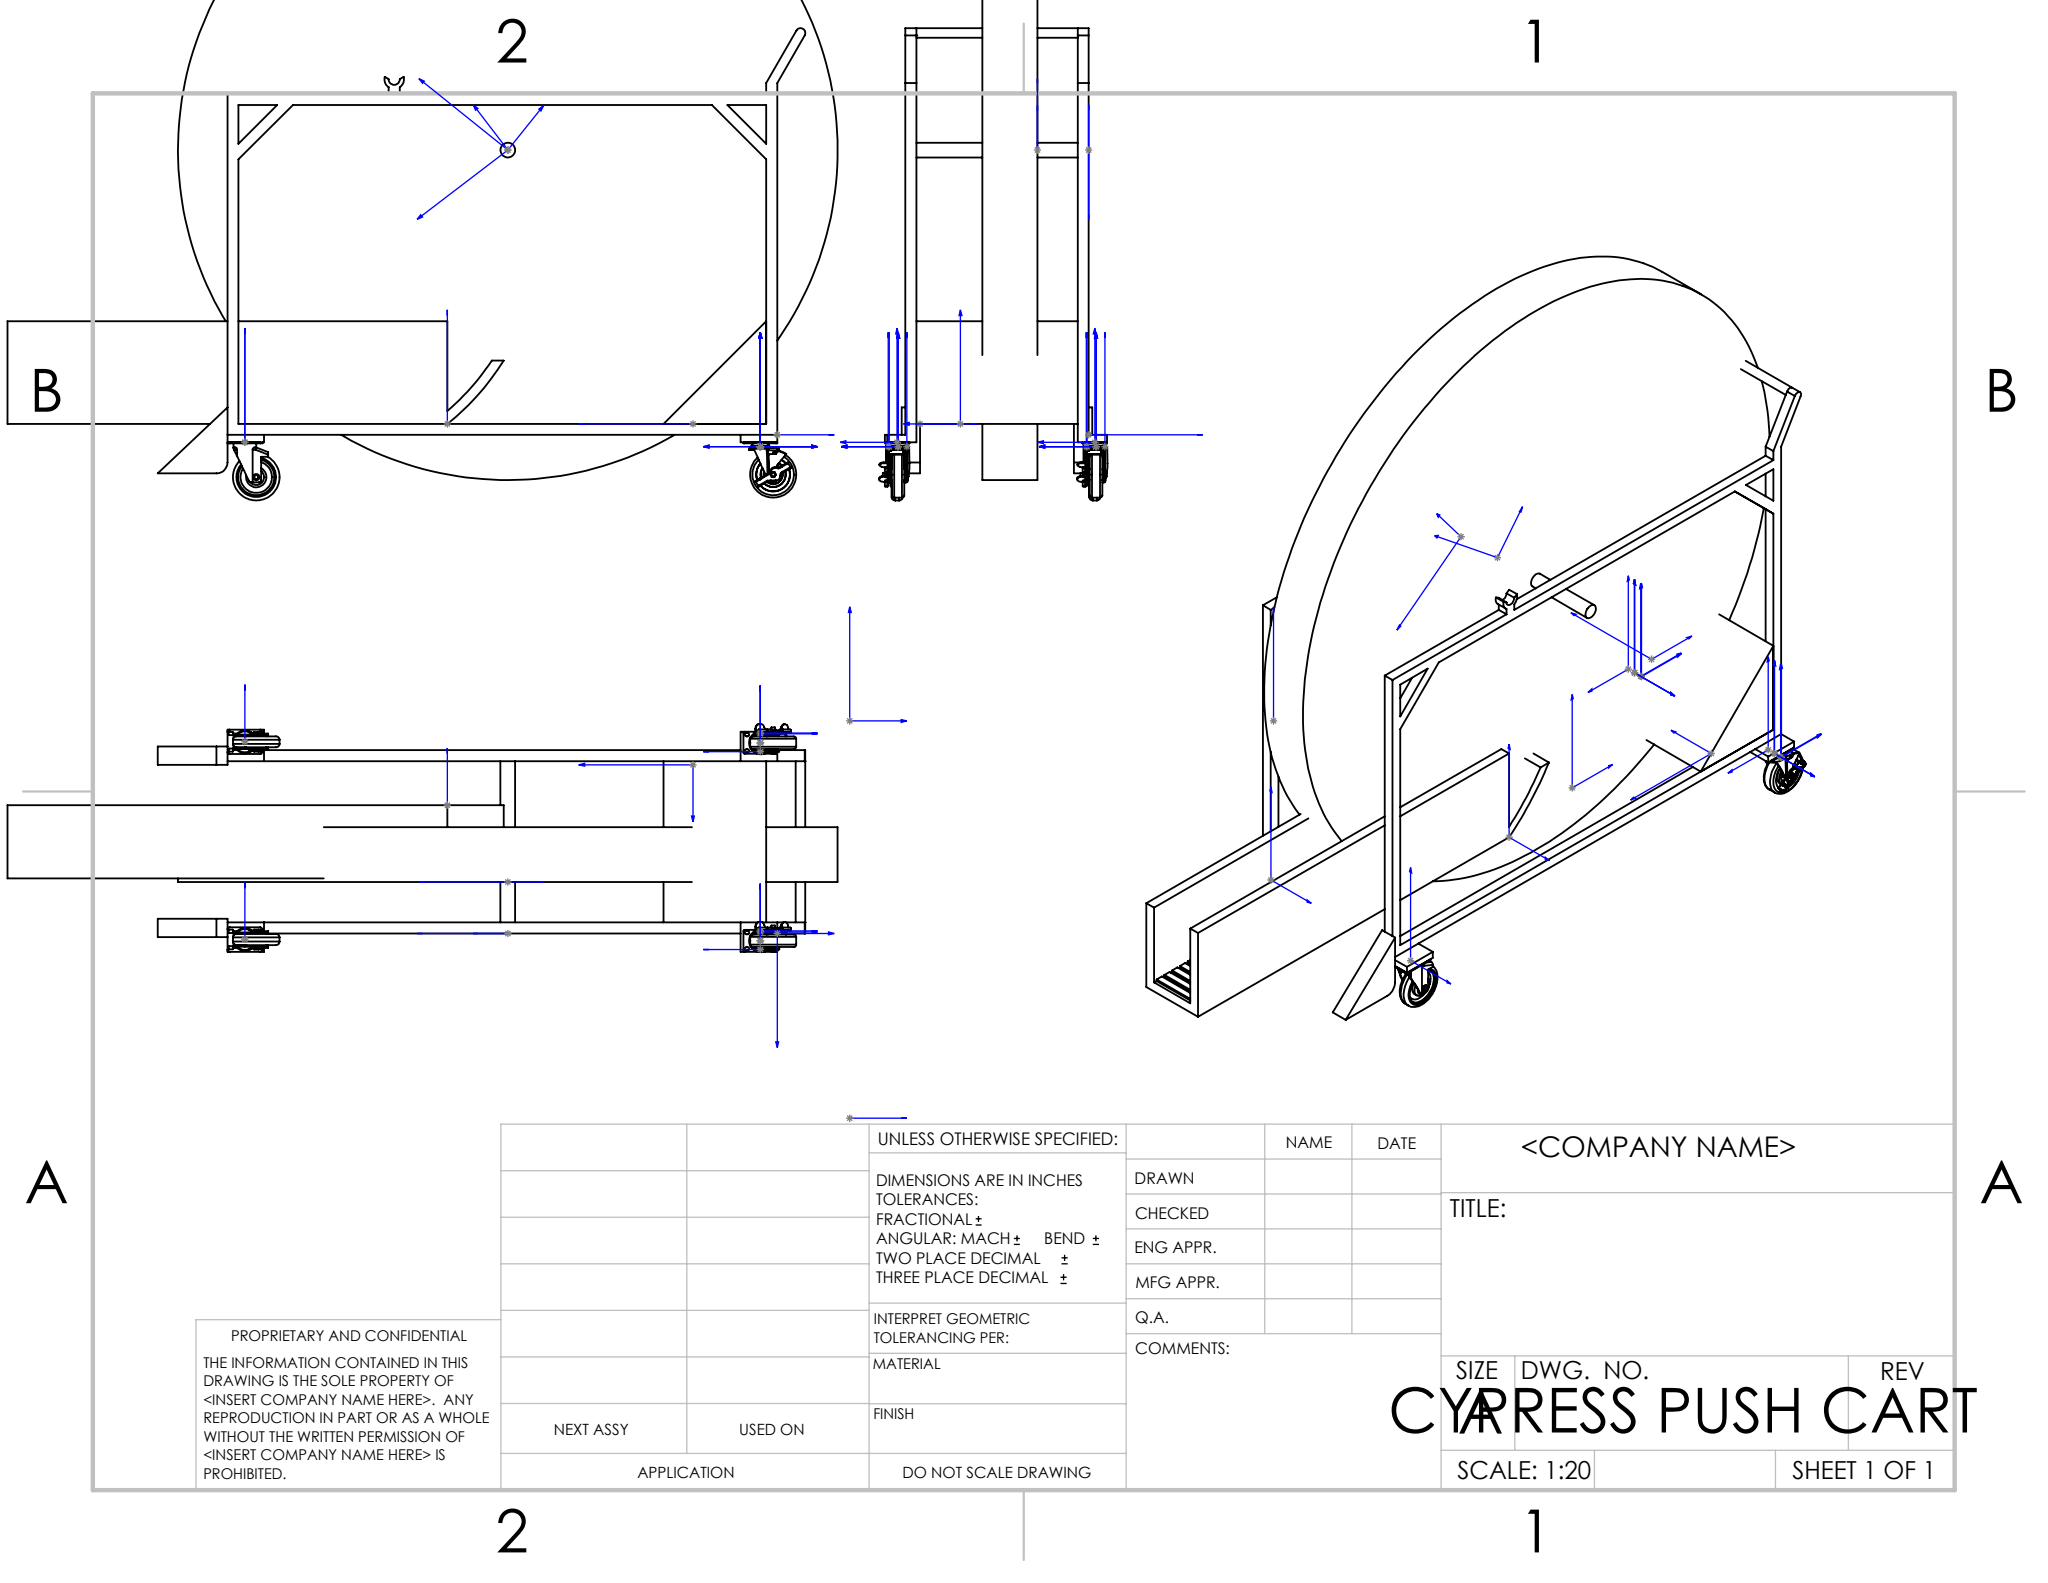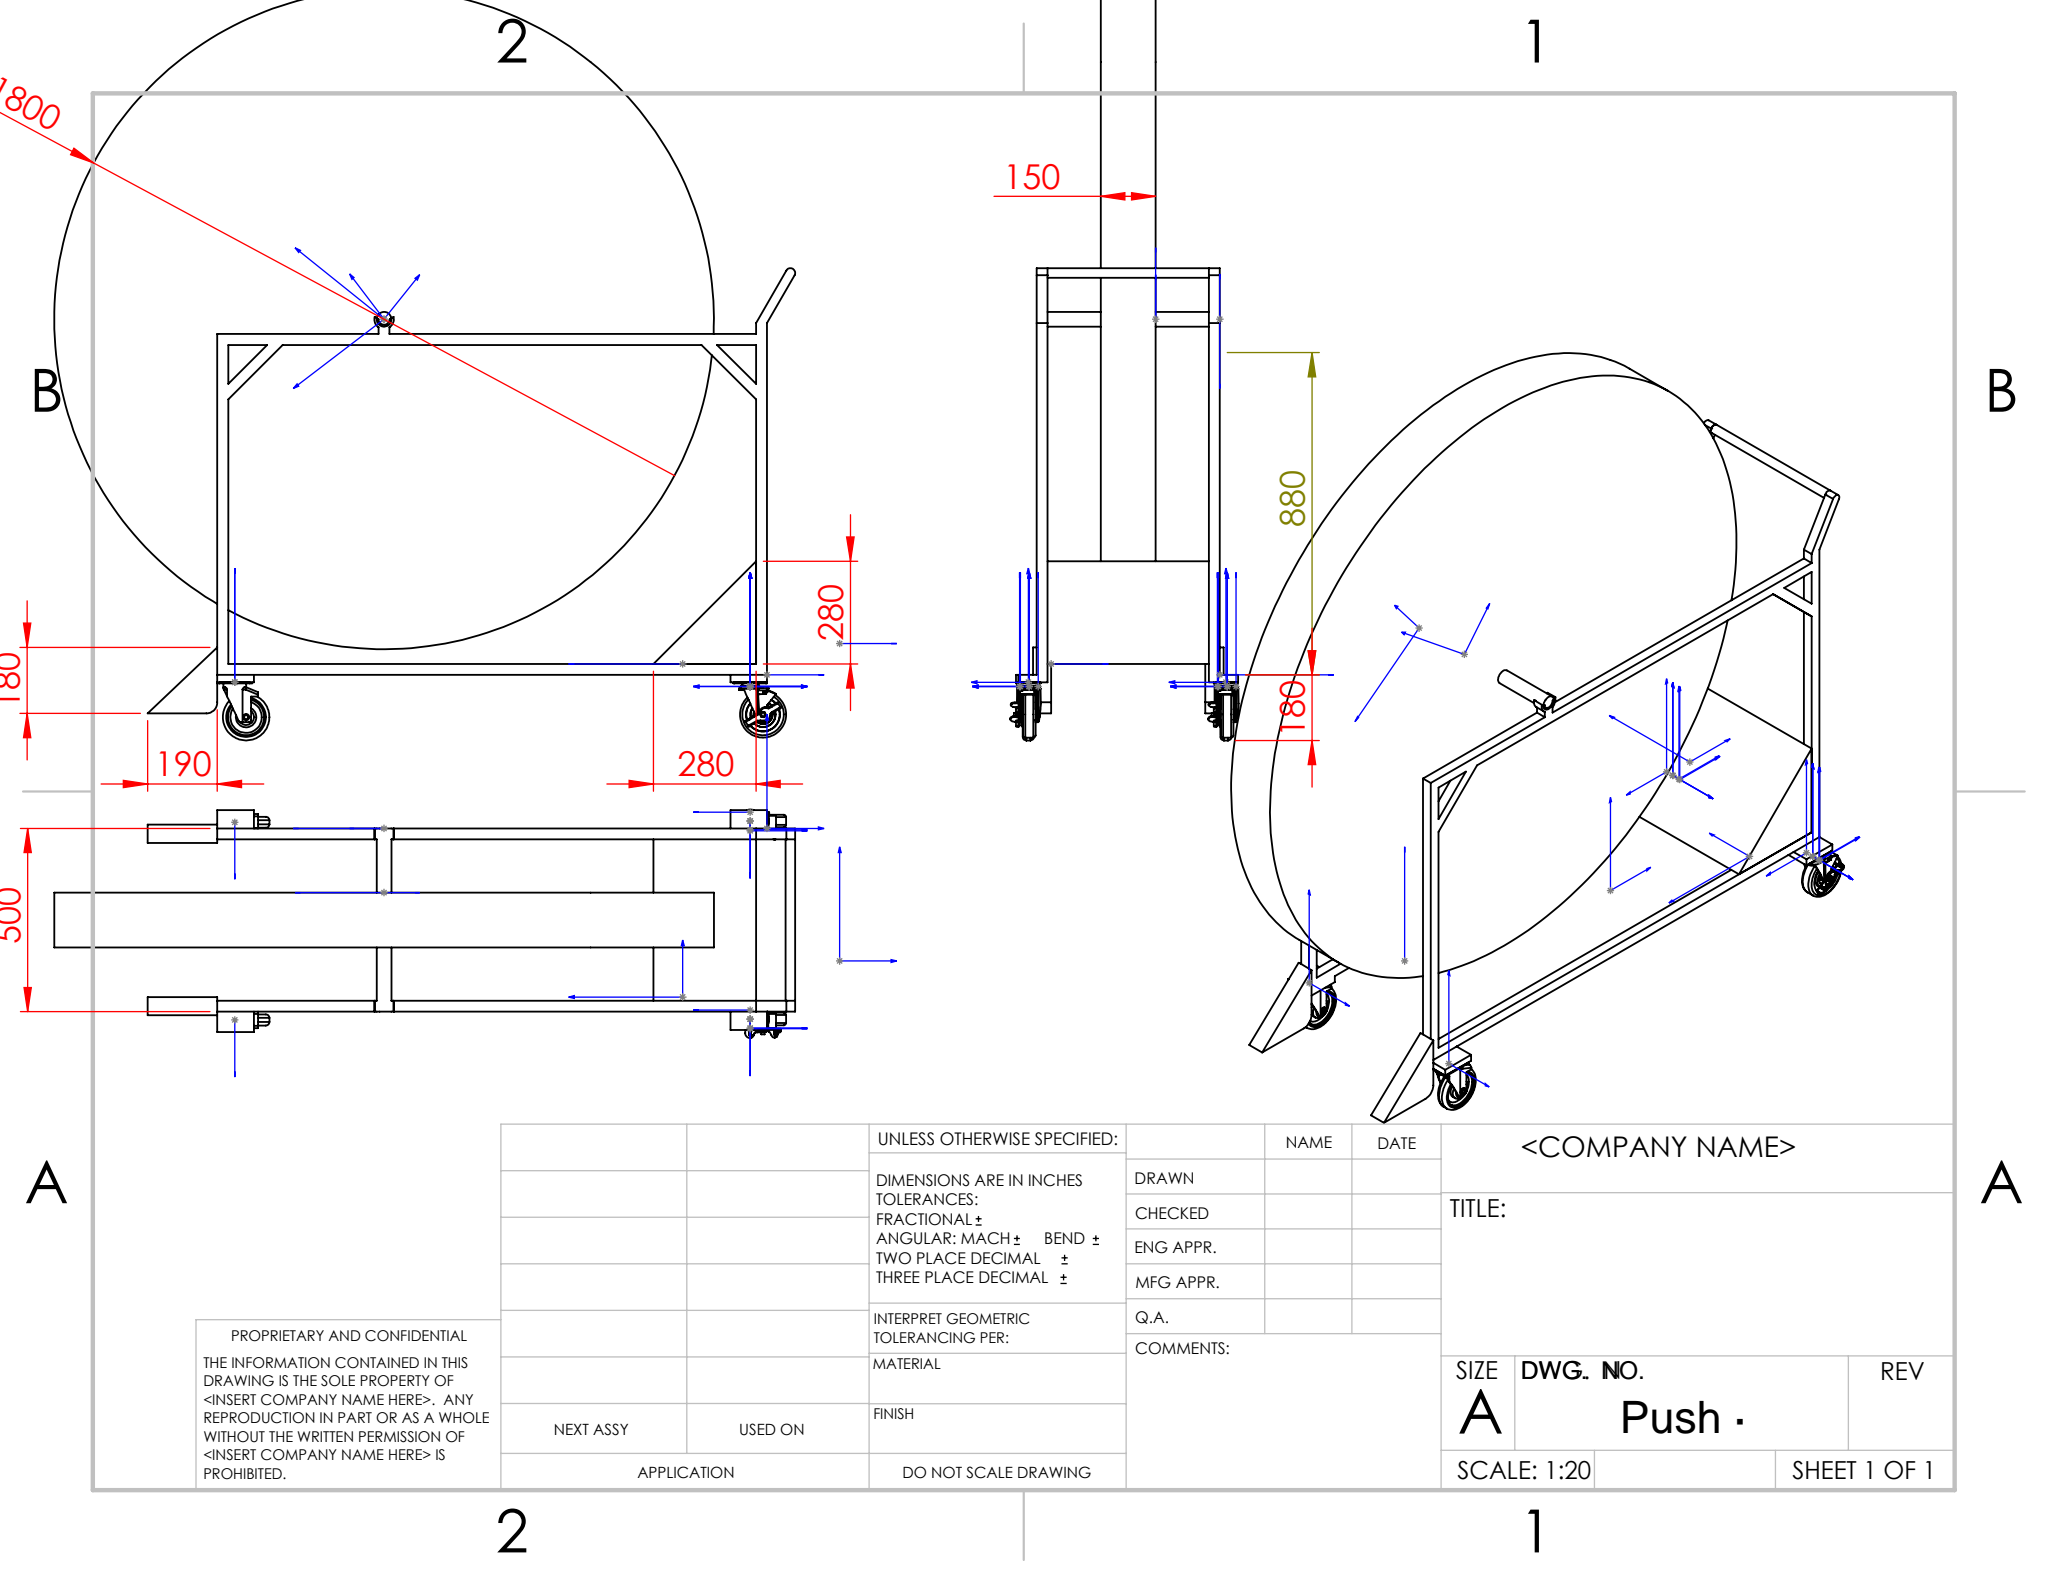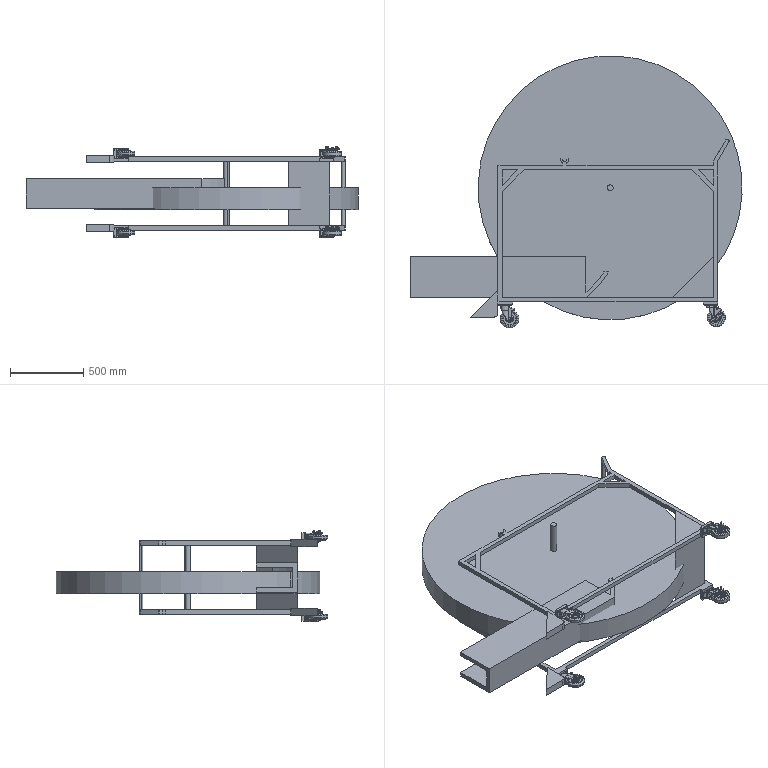Part | SolidWorks | 19 solids | 1176 faces | box 2265 x 1855 x 622.797 mm | volume 442404059 mm3 | plane 661 | cylinder 293 | torus 92 | spline 86 | cone 44 | commonest cylinder face diameters 6.35 x40 12.7 x32 9.017 x24 12.921 x24 17.066 x16 5.08 x12